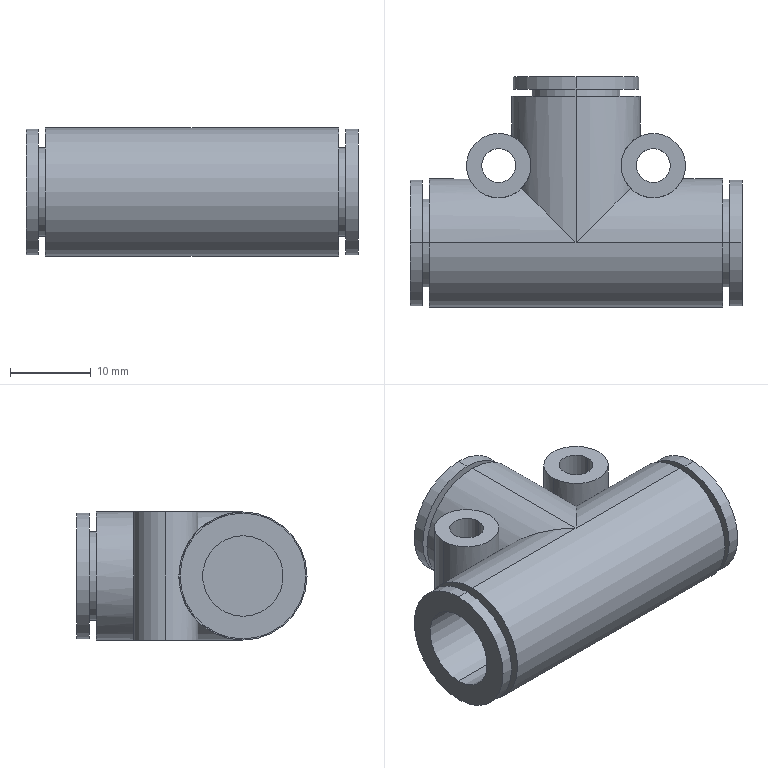Part | SolidWorks | features BaseBody 1 | 1 solid | 47 faces | box 41.2 x 28.55 x 15.9 mm | volume 7852 mm3 | cylinder 31 | plane 16 | commonest cylinder face diameters 10 x6 10.95 x6 15.6 x6 15.9 x5 4.2 x4 8 x4